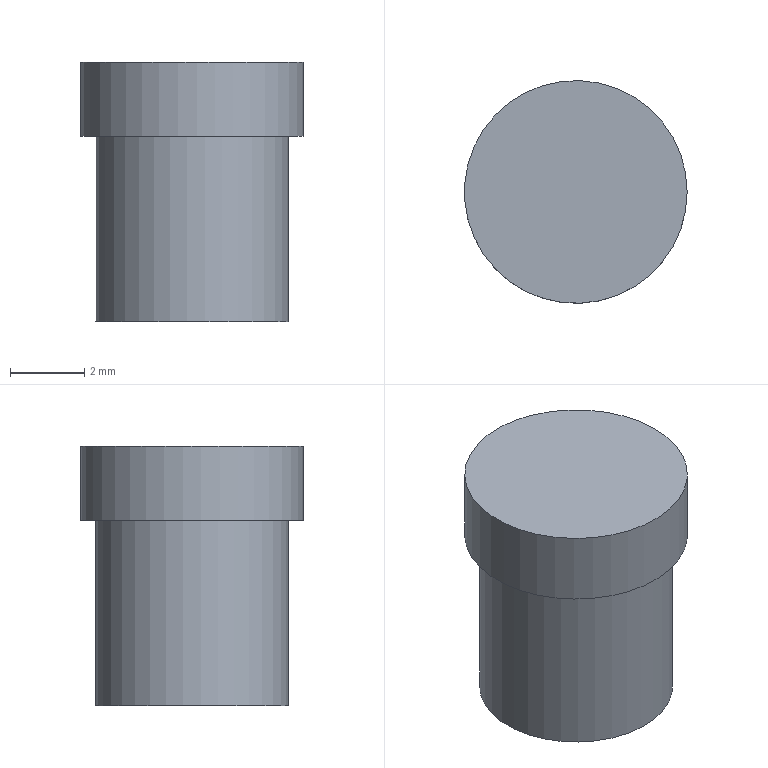Part | NX | features CYLINDER 2, DATUM_CSYS 1 | 1 solid | 5 faces | box 6 x 6 x 7 mm | volume 162.734 mm3 | plane 3 | cylinder 2 | commonest cylinder face diameters 5.2 x1 6 x1
STEP:
#1=CARTESIAN_POINT('',(2.6,0.,0.));
#2=VERTEX_POINT('',#1);
#3=CARTESIAN_POINT('',(0.,0.,0.));
#4=DIRECTION('',(0.,0.,1.));
#5=DIRECTION('',(1.,0.,0.));
#6=AXIS2_PLACEMENT_3D('',#3,#4,#5);
#7=CIRCLE('',#6,2.6);
#8=EDGE_CURVE('',#2,#2,#7,.T.);
#9=ORIENTED_EDGE('',*,*,#8,.F.);
#10=EDGE_LOOP('',(#9));
#11=FACE_BOUND('',#10,.T.);
#12=CARTESIAN_POINT('',(0.,0.,0.));
#13=DIRECTION('',(0.,0.,-1.));
#14=DIRECTION('',(-1.,0.,0.));
#15=AXIS2_PLACEMENT_3D('',#12,#13,#14);
#16=PLANE('',#15);
#17=ADVANCED_FACE('',(#11),#16,.T.);
#18=CARTESIAN_POINT('',(2.6,0.,5.));
#19=VERTEX_POINT('',#18);
#20=CARTESIAN_POINT('',(0.,0.,5.));
#21=DIRECTION('',(0.,0.,-1.));
#22=DIRECTION('',(1.,0.,0.));
#23=AXIS2_PLACEMENT_3D('',#20,#21,#22);
#24=CIRCLE('',#23,2.6);
#25=EDGE_CURVE('',#19,#19,#24,.T.);
#26=ORIENTED_EDGE('',*,*,#25,.T.);
#27=EDGE_LOOP('',(#26));
#28=FACE_BOUND('',#27,.T.);
#29=ORIENTED_EDGE('',*,*,#8,.T.);
#30=EDGE_LOOP('',(#29));
#31=FACE_BOUND('',#30,.T.);
#32=CARTESIAN_POINT('',(0.,0.,0.));
#33=DIRECTION('',(0.,0.,1.));
#34=DIRECTION('',(1.,0.,0.));
#35=AXIS2_PLACEMENT_3D('',#32,#33,#34);
#36=CYLINDRICAL_SURFACE('',#35,2.6);
#37=ADVANCED_FACE('',(#28,#31),#36,.T.);
#38=CARTESIAN_POINT('',(3.,0.,7.));
#39=VERTEX_POINT('',#38);
#40=CARTESIAN_POINT('',(0.,0.,7.));
#41=DIRECTION('',(0.,0.,-1.));
#42=DIRECTION('',(1.,0.,0.));
#43=AXIS2_PLACEMENT_3D('',#40,#41,#42);
#44=CIRCLE('',#43,3.);
#45=EDGE_CURVE('',#39,#39,#44,.T.);
#46=ORIENTED_EDGE('',*,*,#45,.F.);
#47=EDGE_LOOP('',(#46));
#48=FACE_BOUND('',#47,.T.);
#49=CARTESIAN_POINT('',(0.,0.,7.));
#50=DIRECTION('',(0.,0.,1.));
#51=DIRECTION('',(1.,0.,0.));
#52=AXIS2_PLACEMENT_3D('',#49,#50,#51);
#53=PLANE('',#52);
#54=ADVANCED_FACE('',(#48),#53,.T.);
#55=ORIENTED_EDGE('',*,*,#25,.F.);
#56=EDGE_LOOP('',(#55));
#57=FACE_BOUND('',#56,.T.);
#58=CARTESIAN_POINT('',(3.,0.,5.));
#59=VERTEX_POINT('',#58);
#60=CARTESIAN_POINT('',(0.,0.,5.));
#61=DIRECTION('',(0.,0.,1.));
#62=DIRECTION('',(1.,0.,0.));
#63=AXIS2_PLACEMENT_3D('',#60,#61,#62);
#64=CIRCLE('',#63,3.);
#65=EDGE_CURVE('',#59,#59,#64,.T.);
#66=ORIENTED_EDGE('',*,*,#65,.F.);
#67=EDGE_LOOP('',(#66));
#68=FACE_BOUND('',#67,.T.);
#69=CARTESIAN_POINT('',(0.,0.,5.));
#70=DIRECTION('',(0.,0.,-1.));
#71=DIRECTION('',(-1.,0.,0.));
#72=AXIS2_PLACEMENT_3D('',#69,#70,#71);
#73=PLANE('',#72);
#74=ADVANCED_FACE('',(#57,#68),#73,.T.);
#75=ORIENTED_EDGE('',*,*,#45,.T.);
#76=EDGE_LOOP('',(#75));
#77=FACE_BOUND('',#76,.T.);
#78=ORIENTED_EDGE('',*,*,#65,.T.);
#79=EDGE_LOOP('',(#78));
#80=FACE_BOUND('',#79,.T.);
#81=CARTESIAN_POINT('',(0.,0.,5.));
#82=DIRECTION('',(0.,0.,1.));
#83=DIRECTION('',(1.,0.,0.));
#84=AXIS2_PLACEMENT_3D('',#81,#82,#83);
#85=CYLINDRICAL_SURFACE('',#84,3.);
#86=ADVANCED_FACE('',(#77,#80),#85,.T.);
#87=CLOSED_SHELL('',(#17,#37,#54,#74,#86));
#88=MANIFOLD_SOLID_BREP('',#87);
#89=(LENGTH_UNIT()NAMED_UNIT(*)SI_UNIT(.MILLI.,.METRE.));
#90=UNCERTAINTY_MEASURE_WITH_UNIT(LENGTH_MEASURE(0.00001),#89,'','');
#91=(NAMED_UNIT(*)PLANE_ANGLE_UNIT()SI_UNIT($,.RADIAN.));
#92=(NAMED_UNIT(*)SI_UNIT($,.STERADIAN.)SOLID_ANGLE_UNIT());
#93=(GEOMETRIC_REPRESENTATION_CONTEXT(3)GLOBAL_UNCERTAINTY_ASSIGNED_CONTEXT((#90))GLOBAL_UNIT_ASSIGNED_CONTEXT((#89,#91,#92))REPRESENTATION_CONTEXT('',''));
#94=ADVANCED_BREP_SHAPE_REPRESENTATION('',(#88),#93);